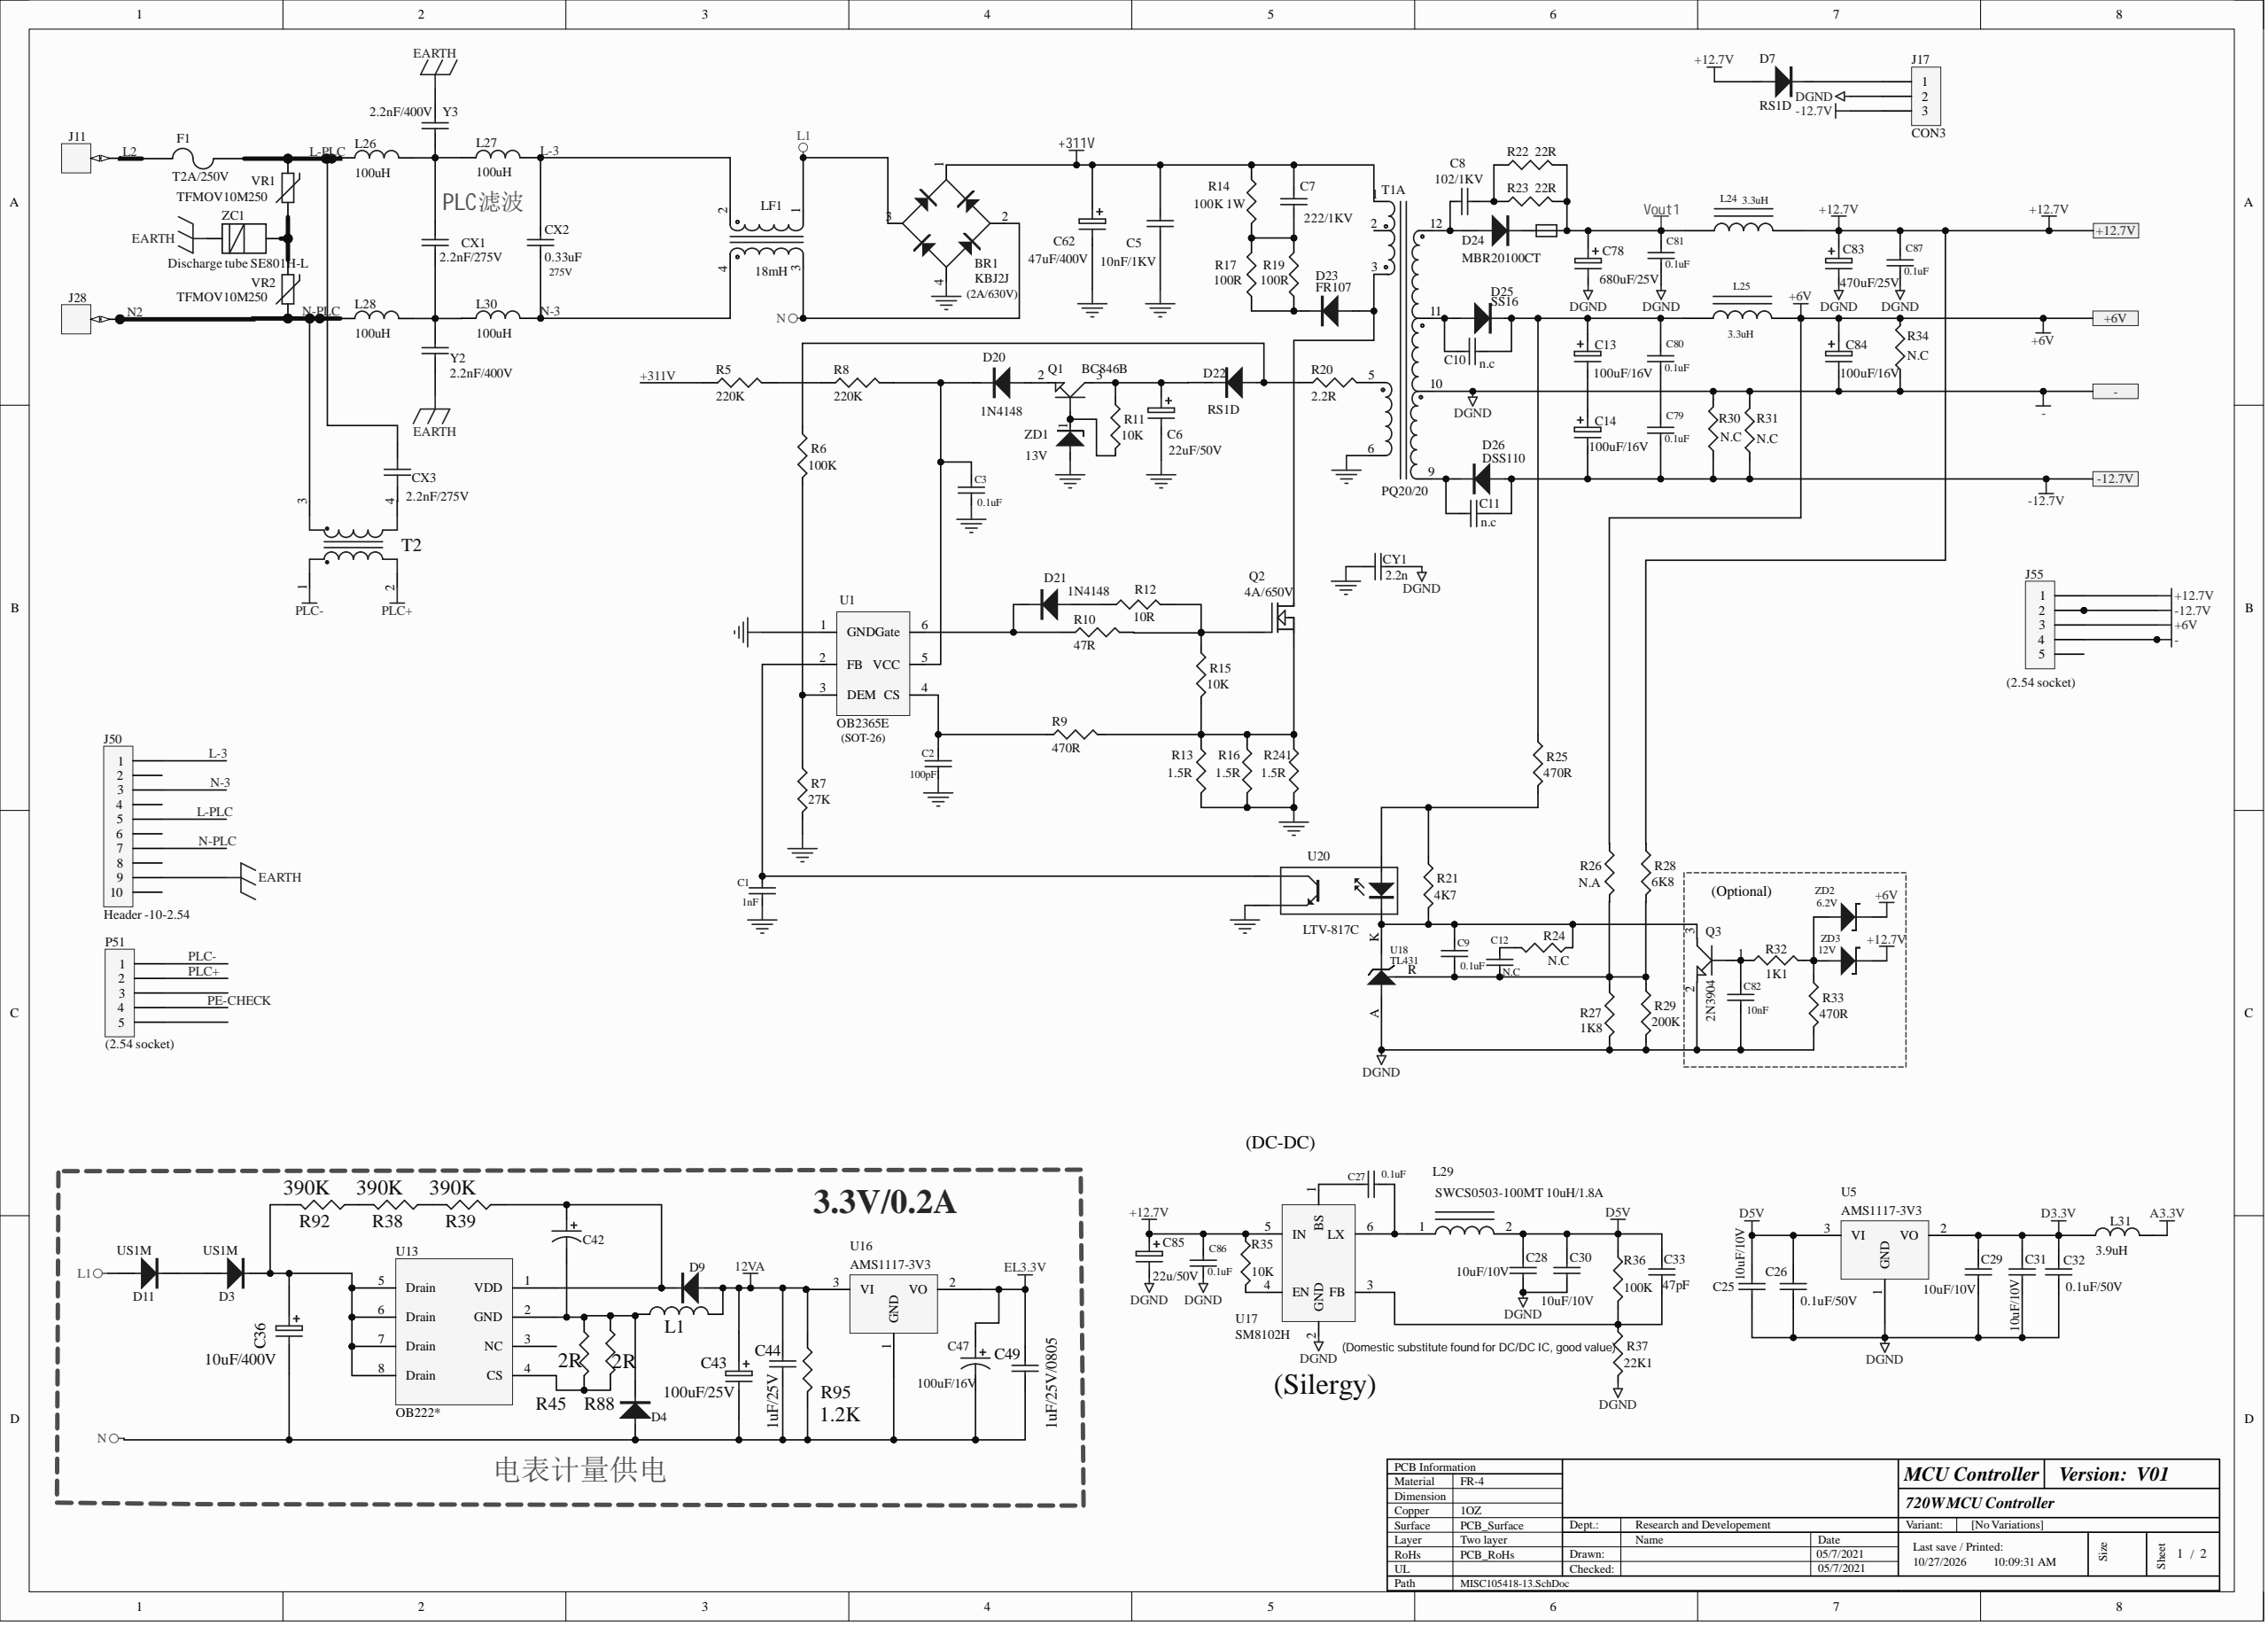Circuit board | Altium Designer | 455 parts | 280 nets | one sheet of the schematic
Parts on this sheet (reference | value | footprint):
BR1 | KBJ2J | BD15.22X4.5(KBP206）RS-2
C1 | 1nF | C0805-T
C2 | 100pF | C0805-T
C3 | 0.1uF | C0805-T
C5 | 10nF/1KV | C1206-T
C6 | 22uF/50V | CE5-P2.5MM-AI-DS
C7 | 222/1KV | CC7.5-P5.0MM-AI-2.5-DS
C8 | 102/1KV | C1206-T
C9 | 0.1uF | C0805-T
C10 | n.c | C1206-T
C11 | n.c | C1206-T
C12 | N.C | C0805-T
C13 | 100uF/16V | CE5-P2.5MM-AI-DS
C14 | 100uF/16V | CE5-P2.5MM-AI-DS
C25 | 10uF/10V | C0805-T
C26 | 0.1uF/50V | C0603-T
C27 | 0.1uF | C0805-T
C28 | 10uF/10V | C0805-T
C29 | 10uF/10V | C0805-T
C30 | 10uF/10V | C0805-T
C31 | 10uF/10V | C0805-T
C32 | 0.1uF/50V | C0603-T
C33 | 47pF | C0805-T
C36 | 10uF/400V | CE10-P5.0MM-AI
C42 | 10uF/50V | CE5-P2.5MM-AI
C43 | 100uF/25V | CE10-P5.0MM-AI
C44 | 1uF/25V | C0805-T
C47 | 100uF/16V | CE5-P2.5MM-AI
C49 | 1uF/25V/0805 | C0805-T
C62 | 47uF/400V | CE18
C78 | 680uF/25V | CE8-P2.5MM-AI-DS
C79 | 0.1uF | C0805-T
C80 | 0.1uF | C0805-T
C81 | 0.1uF | C0805-T
C82 | 10nF | C0805-T
C83 | 470uF/25V | CE8-P2.5MM-AI-DS
C84 | 100uF/16V | CE5-P2.5MM-AI-DS
C85 | 22u/50V | CE6.3-P2.5MM-AI-DS
C86 | 0.1uF | C0805-T
C87 | 0.1uF | C0805-T
CX1 | 2.2nF/275V | CX12.0X6.0-P10
CX2 | 0.33uF | CX10.0X4.0-P7.5
CX3 | 2.2nF/275V | CX12.0X6.0-P10
CY1 | 2.2n | CY7.5X4.7_P10_AI-DS
D3 | US1M | SMA
D4 | MUR406 | SMA
D7 | RS1D | SMA
D9 | MUR406 | SMA
D11 | US1M | SMA
D20 | 1N4148 | SOD-123-T
D21 | 1N4148 | SOD-123-T
D22 | RS1D | SMA-T
D23 | FR107 | SMA-T
D24 | MBR20100CT | TO-220(AKA二极管）
D25 | SS16 | SMA-T
D26 | DSS110 | SMA-T
F1 | T2A/250V | FUSE-TE5
J11 | Terminal | 接线端子（12X9mm）
J17 | CON3 | CON3-3.81
J28 | Terminal | 接线端子（12X9mm）
J50 | Header -10-2.54 | p10-2.54
J55 | (2.54 socket) | P5-2.54
L1 | 1mH  DR8*10 | R0805-T
L24 | 3.3uH | L-DR6-P5.0
L25 | 3.3uH | L-DR6-P5.0
L26 | 100uH | 71453-00013-11 (5X8.3 P:2.5)
L27 | 100uH | 71453-00013-11 (5X8.3 P:2.5)
L28 | 100uH | 71453-00013-11 (5X8.3 P:2.5)
L29 | SWCS0503-100MT 10uH/1.8A | L(8x8x4)-3d
L30 | 100uH | 71453-00013-11 (5X8.3 P:2.5)
L31 | 3.9uH | R0805-T
LF1 | 18mH | UU9.8 - (8.7MM)
P51 | (2.54 socket) | P5-2.54
Q1 | BC846B | SOT-23-T
Q2 | 4A/650V | TO-220((散热片16.5X16mm 厚1.5mm)
Q3 | 2N3904 | SOT-23-T
R5 | 220K | R1206-T
R6 | 100K | R0805-T
R7 | 27K | R0805-T
R8 | 220K | R1206-T
R9 | 470R | R0805-T
R10 | 47R | R1206-T
R11 | 10K | R0805-T
R12 | 10R | R1206-T
R13 | 1.5R | R1206-T
R14 | 100K 1W | R-1W-P5.0-V
R15 | 10K | R0805-T
R16 | 1.5R | R1206-T
R17 | 100R | R1206-T
R19 | 100R | R1206-T
R20 | 2.2R | R1206-T
R21 | 4K7 | R0805-T
R22 | 22R | R1206-T
R23 | 22R | R1206-T
R24 | N.C | R0805-T
R25 | 470R | R0805-T
R26 | N.A | R0805-T
R27 | 1K8 | R0805-T
R28 | 6K8 | R0805-T
R29 | 200K | R0805-T
R30 | N.C | R1206-T
R31 | N.C | R1206-T
R32 | 1K1 | R0805-T
R33 | 470R | R0805-T
R34 | N.C | R1206-T
R35 | 10K | R0805-T
R36 | 100K | R0805-T
R37 | 22K1 | R0805-T
R38 | 390K | R1206-T
R39 | 390K | R1206-T
R45 | 2R | R1206-T
R88 | 2R | R1206-T
R92 | 390K | R1206-T
R95 | 1.2K | R1206-T
R241 | 1.5R | R1206-T
T2 | EFD30 | 变压器
U1 | OB2365E | SOT-23-6-T
U5 | AMS1117-3V3 | SOT-223-T
U13 | OB222* | SO-8-t
U16 | AMS1117-3V3 | SOT-223-T
U17 | SM8102H | SOT-23-6-T
U18 | TL431 | SOT-23((TL431)(A K R)-T
U20 | LTV-817C | OPT-SMT(LTV-817S)
VR1 | TFMOV10M250 | 防雷单元TFMOV10M
VR2 | TFMOV10M250 | 防雷单元TFMOV10M
Y2 | 2.2nF/400V | CY7.5X4.7_P10_AI-DS
Y3 | 2.2nF/400V | CY7.5X4.7_P10_AI-DS
ZC1 | Discharge tube SE801H-L | ZC 8X6.5  P:16.0mm
ZD1 | 13V | SOD-123-T
ZD2 | 6.2V | SOD-123-T
ZD3 | 12V | SOD-123-T
Nets of these parts (net: part-pin ...):
Vout1: C78-1 C81-2 D24-2 L24-1 R22-2 R23-2
PLC-: P51-1 T2-1
PLC+: P51-2 T2-2
PE-CHECK: P51-4
NetVR1_1: VR1-1 VR2-2 ZC1-2
NetR45_2: R45-2 R88-2 U13-4
NetR38_2: R38-2 R92-1
NetR38_1: R38-1 R39-2
NetR35_2: R35-2 U17-4
NetR32_2: R32-2 R33-1 ZD2-1 ZD3-1
NetR21_1: R21-1 R25-2 U20-1
NetR20_2: R20-2
NetR6_2: R6-2 R7-1 U1-3
NetR5_2: R5-2 R8-1
NetQ2_3: Q2-3 R9-2 R13-1 R15-2 R16-1 R241-1
NetQ2_1: Q2-1 R10-2 R12-2 R15-1
NetQ1_1: Q1-1 R11-2 ZD1-2
NetD23_2: D23-2 R17-1 R19-1
NetD23_1: D23-1 Q2-2
NetD22_1: D22-1 R6-1 R20-1
NetD21_2: D21-2 R10-1 U1-6
NetD21_1: D21-1 R12-1
NetD20_1: D20-1 Q1-2
NetD7_2: D7-2 J17-1
NetD3_1: D3-1 D11-2
NetCX3_1: CX3-1 T2-4
NetCX1_2: CX1-2 L26-2 L27-1 Y3-2
NetCX1_1: CX1-1 L28-2 L30-1 Y2-1
NetC82_1: C82-1 Q3-1 R32-1
NetC79_2: C79-2 C80-1
NetC42_2: C42-2 D4-2 L1-1 R45-1 R88-1 U13-2
NetC42_1: C42-1 D9-2 R39-1 U13-1
NetC36_1: C36-1 D3-2 R92-2 U13-5 U13-6 U13-7 U13-8
NetC33_2: C33-2 R36-2 R37-1 U17-3
NetC27_2: C27-2 L29-1 U17-6
NetC27_1: C27-1 U17-1
NetC13_2: C13-2 C14-1
NetC12_1: C12-1 R24-2
NetC11_1: C11-1 D26-2
NetC10_2: C10-2 C13-1 C80-2 D25-2 L25-1 R25-1
NetC10_1: C10-1 D25-1
NetC9_2: C9-2 C12-2 R26-2 R27-1 R28-2 R29-1 U18-R
NetC9_1: C9-1 Q3-3 R21-2 R24-1 U18-K U20-2
NetC8_2: C8-2 R22-1 R23-1
NetC8_1: C8-1 D24-1
NetC7_1: C7-1 R14-2 R17-2 R19-2
NetC6_1: C6-1 D22-2 Q1-3 R11-1
NetC3_1: C3-1 D20-2 R8-2 U1-5
NetC2_1: C2-1 R9-1 U1-4
NetC1_1: C1-1 U1-2 U20-3
N-3: CX2-2 J50-3 L30-2 LF1-4
N2: J28-1 J50-7 L28-1 T2-3 VR2-1
N: BR1-2 C36-2 C43-2 C44-1 C47-2 C49-1 D4-1 LF1-3 R95-2 U16-1
L-PLC: CX3-2 F1-2 J50-5 L26-1 VR1-2
L-3: CX2-1 J50-1 L27-2 LF1-2
L2: F1-1 J11-1
L1: BR1-3 D11-1 LF1-1
GND: BR1-4 C1-2 C2-2 C3-2 C5-2 C6-2 C62-2 CY1-2 R7-2 R13-2 R16-2 R241-2 U1-1 U20-4 ZD1-1
EL3.3V: C47-1 C49-2 U16-2
EARTH: J50-9 Y2-2 Y3-1 ZC1-1
D5V: C25-1 C26-1 C28-1 C30-1 C33-1 L29-2 R36-1 U5-3
D3.3V: C29-1 C31-1 C32-1 L31-1 U5-2
A3.3V: L31-2
-12.7V: C11-2 C14-2 C79-1 D26-1 J17-3 J55-2 R30-1 R31-1
-: C25-2 C26-2 C28-2 C29-2 C30-2 C31-2 C32-2 C78-2 C81-1 C82-2 C83-2 C84-2 C85-2 C86-1 C87-1 CY1-1 J17-2 J55-4 Q3-2 R27-2 R29-2 R30-2 R31-2 R33-2 R34-1 R37-2 U5-1 U17-2 U18-A
+311V: BR1-1 C5-1 C7-2 C62-1 R5-1 R14-1
+12.7V: C83-1 C85-1 C86-2 C87-2 D7-1 J55-1 L24-2 R28-1 R35-1 U17-5 ZD3-2
+6V: C84-1 J55-3 L25-2 R26-1 R34-2 ZD2-2
12VA: C43-1 C44-2 D9-1 L1-2 R95-1 U16-3